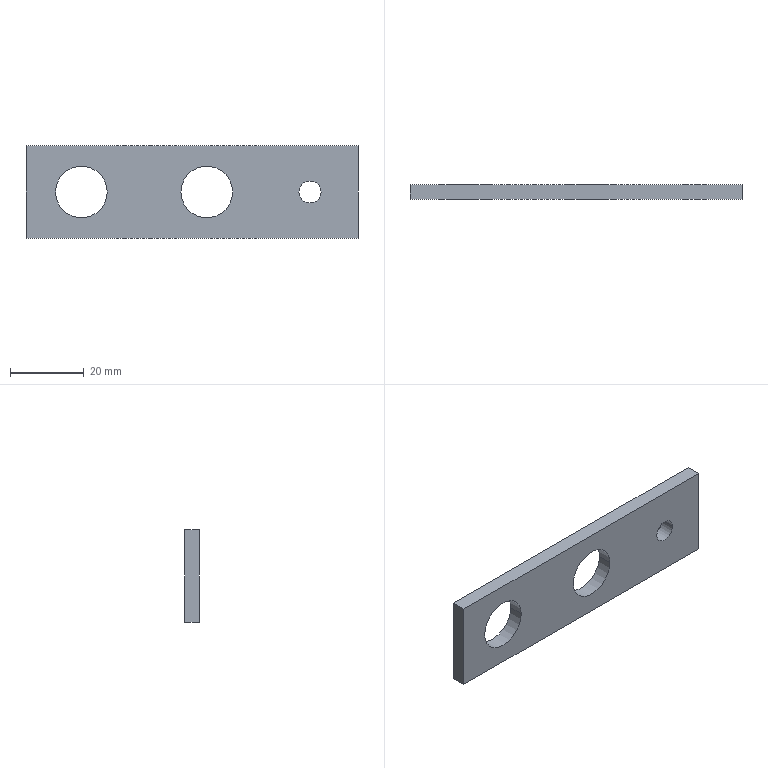Part | STEP file | Connecting plate 2 | 1 solid | 12 faces | box 90 x 4 x 25 mm | volume 7655 mm3 | cylinder 6 | plane 6 | commonest cylinder face diameters 14 x4 6 x2
STEP:
#1=CARTESIAN_POINT('',(-68.,0.,12.5));
#2=VERTEX_POINT('',#1);
#3=CARTESIAN_POINT('',(-82.,0.,12.5));
#4=VERTEX_POINT('',#3);
#5=CARTESIAN_POINT('',(-75.,0.,12.5));
#6=DIRECTION('',(0.,1.,0.));
#7=DIRECTION('',(1.,0.,0.));
#8=AXIS2_PLACEMENT_3D('',#5,#6,#7);
#9=CIRCLE('',#8,7.);
#10=EDGE_CURVE('',#2,#4,#9,.T.);
#11=ORIENTED_EDGE('',*,*,#10,.F.);
#12=CARTESIAN_POINT('',(-68.,4.,12.5));
#13=VERTEX_POINT('',#12);
#14=CARTESIAN_POINT('',(-68.,-0.001,12.5));
#15=DIRECTION('',(0.,1.,0.));
#16=VECTOR('',#15,1000.);
#17=LINE('',#14,#16);
#18=EDGE_CURVE('',#2,#13,#17,.T.);
#19=ORIENTED_EDGE('',*,*,#18,.T.);
#20=CARTESIAN_POINT('',(-82.,4.,12.5));
#21=VERTEX_POINT('',#20);
#22=CARTESIAN_POINT('',(-75.,4.,12.5));
#23=DIRECTION('',(0.,1.,0.));
#24=DIRECTION('',(-1.,0.,0.));
#25=AXIS2_PLACEMENT_3D('',#22,#23,#24);
#26=CIRCLE('',#25,7.);
#27=EDGE_CURVE('',#13,#21,#26,.T.);
#28=ORIENTED_EDGE('',*,*,#27,.T.);
#29=CARTESIAN_POINT('',(-82.,-0.001,12.5));
#30=DIRECTION('',(0.,1.,0.));
#31=VECTOR('',#30,1000.);
#32=LINE('',#29,#31);
#33=EDGE_CURVE('',#4,#21,#32,.T.);
#34=ORIENTED_EDGE('',*,*,#33,.F.);
#35=EDGE_LOOP('',(#11,#19,#28,#34));
#36=FACE_OUTER_BOUND('',#35,.T.);
#37=CARTESIAN_POINT('',(-75.,-0.001,12.5));
#38=DIRECTION('',(0.,1.,0.));
#39=DIRECTION('',(-1.,0.,0.));
#40=AXIS2_PLACEMENT_3D('',#37,#38,#39);
#41=CYLINDRICAL_SURFACE('',#40,7.);
#42=ADVANCED_FACE('',(#36),#41,.F.);
#43=CARTESIAN_POINT('',(-10.,0.,12.5));
#44=VERTEX_POINT('',#43);
#45=CARTESIAN_POINT('',(-16.,0.,12.5));
#46=VERTEX_POINT('',#45);
#47=CARTESIAN_POINT('',(-13.,0.,12.5));
#48=DIRECTION('',(0.,1.,0.));
#49=DIRECTION('',(1.,0.,0.));
#50=AXIS2_PLACEMENT_3D('',#47,#48,#49);
#51=CIRCLE('',#50,3.);
#52=EDGE_CURVE('',#44,#46,#51,.T.);
#53=ORIENTED_EDGE('',*,*,#52,.F.);
#54=CARTESIAN_POINT('',(-10.,4.,12.5));
#55=VERTEX_POINT('',#54);
#56=CARTESIAN_POINT('',(-10.,-0.001,12.5));
#57=DIRECTION('',(0.,1.,0.));
#58=VECTOR('',#57,1000.);
#59=LINE('',#56,#58);
#60=EDGE_CURVE('',#44,#55,#59,.T.);
#61=ORIENTED_EDGE('',*,*,#60,.T.);
#62=CARTESIAN_POINT('',(-16.,4.,12.5));
#63=VERTEX_POINT('',#62);
#64=CARTESIAN_POINT('',(-13.,4.,12.5));
#65=DIRECTION('',(0.,1.,0.));
#66=DIRECTION('',(-1.,0.,0.));
#67=AXIS2_PLACEMENT_3D('',#64,#65,#66);
#68=CIRCLE('',#67,3.);
#69=EDGE_CURVE('',#55,#63,#68,.T.);
#70=ORIENTED_EDGE('',*,*,#69,.T.);
#71=CARTESIAN_POINT('',(-16.,-0.001,12.5));
#72=DIRECTION('',(0.,1.,0.));
#73=VECTOR('',#72,1000.);
#74=LINE('',#71,#73);
#75=EDGE_CURVE('',#46,#63,#74,.T.);
#76=ORIENTED_EDGE('',*,*,#75,.F.);
#77=EDGE_LOOP('',(#53,#61,#70,#76));
#78=FACE_OUTER_BOUND('',#77,.T.);
#79=CARTESIAN_POINT('',(-13.,-0.001,12.5));
#80=DIRECTION('',(0.,1.,0.));
#81=DIRECTION('',(-1.,0.,0.));
#82=AXIS2_PLACEMENT_3D('',#79,#80,#81);
#83=CYLINDRICAL_SURFACE('',#82,3.);
#84=ADVANCED_FACE('',(#78),#83,.F.);
#85=CARTESIAN_POINT('',(-34.,0.,12.5));
#86=VERTEX_POINT('',#85);
#87=CARTESIAN_POINT('',(-48.,0.,12.5));
#88=VERTEX_POINT('',#87);
#89=CARTESIAN_POINT('',(-41.,0.,12.5));
#90=DIRECTION('',(0.,1.,0.));
#91=DIRECTION('',(1.,0.,0.));
#92=AXIS2_PLACEMENT_3D('',#89,#90,#91);
#93=CIRCLE('',#92,7.);
#94=EDGE_CURVE('',#86,#88,#93,.T.);
#95=ORIENTED_EDGE('',*,*,#94,.F.);
#96=CARTESIAN_POINT('',(-34.,4.,12.5));
#97=VERTEX_POINT('',#96);
#98=CARTESIAN_POINT('',(-34.,-0.001,12.5));
#99=DIRECTION('',(0.,1.,0.));
#100=VECTOR('',#99,1000.);
#101=LINE('',#98,#100);
#102=EDGE_CURVE('',#86,#97,#101,.T.);
#103=ORIENTED_EDGE('',*,*,#102,.T.);
#104=CARTESIAN_POINT('',(-48.,4.,12.5));
#105=VERTEX_POINT('',#104);
#106=CARTESIAN_POINT('',(-41.,4.,12.5));
#107=DIRECTION('',(0.,1.,0.));
#108=DIRECTION('',(-1.,0.,0.));
#109=AXIS2_PLACEMENT_3D('',#106,#107,#108);
#110=CIRCLE('',#109,7.);
#111=EDGE_CURVE('',#97,#105,#110,.T.);
#112=ORIENTED_EDGE('',*,*,#111,.T.);
#113=CARTESIAN_POINT('',(-48.,-0.001,12.5));
#114=DIRECTION('',(0.,1.,0.));
#115=VECTOR('',#114,1000.);
#116=LINE('',#113,#115);
#117=EDGE_CURVE('',#88,#105,#116,.T.);
#118=ORIENTED_EDGE('',*,*,#117,.F.);
#119=EDGE_LOOP('',(#95,#103,#112,#118));
#120=FACE_OUTER_BOUND('',#119,.T.);
#121=CARTESIAN_POINT('',(-41.,-0.001,12.5));
#122=DIRECTION('',(0.,1.,0.));
#123=DIRECTION('',(-1.,0.,0.));
#124=AXIS2_PLACEMENT_3D('',#121,#122,#123);
#125=CYLINDRICAL_SURFACE('',#124,7.);
#126=ADVANCED_FACE('',(#120),#125,.F.);
#127=CARTESIAN_POINT('',(-75.,4.,12.5));
#128=DIRECTION('',(0.,1.,0.));
#129=DIRECTION('',(-1.,0.,0.));
#130=AXIS2_PLACEMENT_3D('',#127,#128,#129);
#131=CIRCLE('',#130,7.);
#132=EDGE_CURVE('',#21,#13,#131,.T.);
#133=ORIENTED_EDGE('',*,*,#132,.F.);
#134=ORIENTED_EDGE('',*,*,#27,.F.);
#135=EDGE_LOOP('',(#133,#134));
#136=FACE_BOUND('',#135,.T.);
#137=CARTESIAN_POINT('',(-13.,4.,12.5));
#138=DIRECTION('',(0.,1.,0.));
#139=DIRECTION('',(-1.,0.,0.));
#140=AXIS2_PLACEMENT_3D('',#137,#138,#139);
#141=CIRCLE('',#140,3.);
#142=EDGE_CURVE('',#63,#55,#141,.T.);
#143=ORIENTED_EDGE('',*,*,#142,.F.);
#144=ORIENTED_EDGE('',*,*,#69,.F.);
#145=EDGE_LOOP('',(#143,#144));
#146=FACE_BOUND('',#145,.T.);
#147=CARTESIAN_POINT('',(-41.,4.,12.5));
#148=DIRECTION('',(0.,1.,0.));
#149=DIRECTION('',(-1.,0.,0.));
#150=AXIS2_PLACEMENT_3D('',#147,#148,#149);
#151=CIRCLE('',#150,7.);
#152=EDGE_CURVE('',#105,#97,#151,.T.);
#153=ORIENTED_EDGE('',*,*,#152,.F.);
#154=ORIENTED_EDGE('',*,*,#111,.F.);
#155=EDGE_LOOP('',(#153,#154));
#156=FACE_BOUND('',#155,.T.);
#157=CARTESIAN_POINT('',(0.,4.,0.));
#158=VERTEX_POINT('',#157);
#159=CARTESIAN_POINT('',(-90.,4.,0.));
#160=VERTEX_POINT('',#159);
#161=CARTESIAN_POINT('',(0.,4.,0.));
#162=DIRECTION('',(-1.,0.,0.));
#163=VECTOR('',#162,1000.);
#164=LINE('',#161,#163);
#165=EDGE_CURVE('',#158,#160,#164,.T.);
#166=ORIENTED_EDGE('',*,*,#165,.T.);
#167=CARTESIAN_POINT('',(-90.,4.,25.));
#168=VERTEX_POINT('',#167);
#169=CARTESIAN_POINT('',(-90.,4.,25.));
#170=DIRECTION('',(0.,0.,-1.));
#171=VECTOR('',#170,1000.);
#172=LINE('',#169,#171);
#173=EDGE_CURVE('',#168,#160,#172,.T.);
#174=ORIENTED_EDGE('',*,*,#173,.F.);
#175=CARTESIAN_POINT('',(0.,4.,25.));
#176=VERTEX_POINT('',#175);
#177=CARTESIAN_POINT('',(0.,4.,25.));
#178=DIRECTION('',(-1.,0.,0.));
#179=VECTOR('',#178,1000.);
#180=LINE('',#177,#179);
#181=EDGE_CURVE('',#176,#168,#180,.T.);
#182=ORIENTED_EDGE('',*,*,#181,.F.);
#183=CARTESIAN_POINT('',(0.,4.,25.));
#184=DIRECTION('',(0.,0.,-1.));
#185=VECTOR('',#184,1000.);
#186=LINE('',#183,#185);
#187=EDGE_CURVE('',#176,#158,#186,.T.);
#188=ORIENTED_EDGE('',*,*,#187,.T.);
#189=EDGE_LOOP('',(#166,#174,#182,#188));
#190=FACE_OUTER_BOUND('',#189,.T.);
#191=CARTESIAN_POINT('',(0.,4.,25.));
#192=DIRECTION('',(0.,-1.,0.));
#193=DIRECTION('',(1.,0.,0.));
#194=AXIS2_PLACEMENT_3D('',#191,#192,#193);
#195=PLANE('',#194);
#196=ADVANCED_FACE('',(#136,#146,#156,#190),#195,.F.);
#197=CARTESIAN_POINT('',(-90.,0.,0.));
#198=VERTEX_POINT('',#197);
#199=CARTESIAN_POINT('',(-90.,0.,0.));
#200=DIRECTION('',(0.,1.,0.));
#201=VECTOR('',#200,1000.);
#202=LINE('',#199,#201);
#203=EDGE_CURVE('',#198,#160,#202,.T.);
#204=ORIENTED_EDGE('',*,*,#203,.F.);
#205=CARTESIAN_POINT('',(-90.,0.,25.));
#206=VERTEX_POINT('',#205);
#207=CARTESIAN_POINT('',(-90.,0.,25.));
#208=DIRECTION('',(0.,0.,-1.));
#209=VECTOR('',#208,1000.);
#210=LINE('',#207,#209);
#211=EDGE_CURVE('',#206,#198,#210,.T.);
#212=ORIENTED_EDGE('',*,*,#211,.F.);
#213=CARTESIAN_POINT('',(-90.,0.,25.));
#214=DIRECTION('',(0.,1.,0.));
#215=VECTOR('',#214,1000.);
#216=LINE('',#213,#215);
#217=EDGE_CURVE('',#206,#168,#216,.T.);
#218=ORIENTED_EDGE('',*,*,#217,.T.);
#219=ORIENTED_EDGE('',*,*,#173,.T.);
#220=EDGE_LOOP('',(#204,#212,#218,#219));
#221=FACE_OUTER_BOUND('',#220,.T.);
#222=CARTESIAN_POINT('',(-90.,0.,25.));
#223=DIRECTION('',(-1.,0.,0.));
#224=DIRECTION('',(0.,0.,1.));
#225=AXIS2_PLACEMENT_3D('',#222,#223,#224);
#226=PLANE('',#225);
#227=ADVANCED_FACE('',(#221),#226,.T.);
#228=CARTESIAN_POINT('',(-75.,0.,12.5));
#229=DIRECTION('',(0.,1.,0.));
#230=DIRECTION('',(1.,0.,0.));
#231=AXIS2_PLACEMENT_3D('',#228,#229,#230);
#232=CIRCLE('',#231,7.);
#233=EDGE_CURVE('',#4,#2,#232,.T.);
#234=ORIENTED_EDGE('',*,*,#233,.T.);
#235=ORIENTED_EDGE('',*,*,#10,.T.);
#236=EDGE_LOOP('',(#234,#235));
#237=FACE_BOUND('',#236,.T.);
#238=CARTESIAN_POINT('',(-13.,0.,12.5));
#239=DIRECTION('',(0.,1.,0.));
#240=DIRECTION('',(1.,0.,0.));
#241=AXIS2_PLACEMENT_3D('',#238,#239,#240);
#242=CIRCLE('',#241,3.);
#243=EDGE_CURVE('',#46,#44,#242,.T.);
#244=ORIENTED_EDGE('',*,*,#243,.T.);
#245=ORIENTED_EDGE('',*,*,#52,.T.);
#246=EDGE_LOOP('',(#244,#245));
#247=FACE_BOUND('',#246,.T.);
#248=CARTESIAN_POINT('',(-41.,0.,12.5));
#249=DIRECTION('',(0.,1.,0.));
#250=DIRECTION('',(1.,0.,0.));
#251=AXIS2_PLACEMENT_3D('',#248,#249,#250);
#252=CIRCLE('',#251,7.);
#253=EDGE_CURVE('',#88,#86,#252,.T.);
#254=ORIENTED_EDGE('',*,*,#253,.T.);
#255=ORIENTED_EDGE('',*,*,#94,.T.);
#256=EDGE_LOOP('',(#254,#255));
#257=FACE_BOUND('',#256,.T.);
#258=CARTESIAN_POINT('',(0.,0.,0.));
#259=VERTEX_POINT('',#258);
#260=CARTESIAN_POINT('',(0.,0.,0.));
#261=DIRECTION('',(-1.,0.,0.));
#262=VECTOR('',#261,1000.);
#263=LINE('',#260,#262);
#264=EDGE_CURVE('',#259,#198,#263,.T.);
#265=ORIENTED_EDGE('',*,*,#264,.F.);
#266=CARTESIAN_POINT('',(0.,0.,25.));
#267=VERTEX_POINT('',#266);
#268=CARTESIAN_POINT('',(0.,0.,25.));
#269=DIRECTION('',(0.,0.,-1.));
#270=VECTOR('',#269,1000.);
#271=LINE('',#268,#270);
#272=EDGE_CURVE('',#267,#259,#271,.T.);
#273=ORIENTED_EDGE('',*,*,#272,.F.);
#274=CARTESIAN_POINT('',(0.,0.,25.));
#275=DIRECTION('',(-1.,0.,0.));
#276=VECTOR('',#275,1000.);
#277=LINE('',#274,#276);
#278=EDGE_CURVE('',#267,#206,#277,.T.);
#279=ORIENTED_EDGE('',*,*,#278,.T.);
#280=ORIENTED_EDGE('',*,*,#211,.T.);
#281=EDGE_LOOP('',(#265,#273,#279,#280));
#282=FACE_OUTER_BOUND('',#281,.T.);
#283=CARTESIAN_POINT('',(0.,0.,25.));
#284=DIRECTION('',(0.,-1.,0.));
#285=DIRECTION('',(1.,0.,0.));
#286=AXIS2_PLACEMENT_3D('',#283,#284,#285);
#287=PLANE('',#286);
#288=ADVANCED_FACE('',(#237,#247,#257,#282),#287,.T.);
#289=CARTESIAN_POINT('',(0.,4.,0.));
#290=DIRECTION('',(0.,-1.,0.));
#291=VECTOR('',#290,1000.);
#292=LINE('',#289,#291);
#293=EDGE_CURVE('',#158,#259,#292,.T.);
#294=ORIENTED_EDGE('',*,*,#293,.F.);
#295=ORIENTED_EDGE('',*,*,#187,.F.);
#296=CARTESIAN_POINT('',(0.,4.,25.));
#297=DIRECTION('',(0.,-1.,0.));
#298=VECTOR('',#297,1000.);
#299=LINE('',#296,#298);
#300=EDGE_CURVE('',#176,#267,#299,.T.);
#301=ORIENTED_EDGE('',*,*,#300,.T.);
#302=ORIENTED_EDGE('',*,*,#272,.T.);
#303=EDGE_LOOP('',(#294,#295,#301,#302));
#304=FACE_OUTER_BOUND('',#303,.T.);
#305=CARTESIAN_POINT('',(0.,4.,25.));
#306=DIRECTION('',(1.,0.,0.));
#307=DIRECTION('',(0.,1.,0.));
#308=AXIS2_PLACEMENT_3D('',#305,#306,#307);
#309=PLANE('',#308);
#310=ADVANCED_FACE('',(#304),#309,.T.);
#311=ORIENTED_EDGE('',*,*,#181,.T.);
#312=ORIENTED_EDGE('',*,*,#217,.F.);
#313=ORIENTED_EDGE('',*,*,#278,.F.);
#314=ORIENTED_EDGE('',*,*,#300,.F.);
#315=EDGE_LOOP('',(#311,#312,#313,#314));
#316=FACE_OUTER_BOUND('',#315,.T.);
#317=CARTESIAN_POINT('',(0.,0.,25.));
#318=DIRECTION('',(0.,0.,-1.));
#319=DIRECTION('',(-1.,0.,0.));
#320=AXIS2_PLACEMENT_3D('',#317,#318,#319);
#321=PLANE('',#320);
#322=ADVANCED_FACE('',(#316),#321,.F.);
#323=ORIENTED_EDGE('',*,*,#165,.F.);
#324=ORIENTED_EDGE('',*,*,#293,.T.);
#325=ORIENTED_EDGE('',*,*,#264,.T.);
#326=ORIENTED_EDGE('',*,*,#203,.T.);
#327=EDGE_LOOP('',(#323,#324,#325,#326));
#328=FACE_OUTER_BOUND('',#327,.T.);
#329=CARTESIAN_POINT('',(0.,0.,0.));
#330=DIRECTION('',(0.,0.,-1.));
#331=DIRECTION('',(-1.,0.,0.));
#332=AXIS2_PLACEMENT_3D('',#329,#330,#331);
#333=PLANE('',#332);
#334=ADVANCED_FACE('',(#328),#333,.T.);
#335=ORIENTED_EDGE('',*,*,#102,.F.);
#336=ORIENTED_EDGE('',*,*,#253,.F.);
#337=ORIENTED_EDGE('',*,*,#117,.T.);
#338=ORIENTED_EDGE('',*,*,#152,.T.);
#339=EDGE_LOOP('',(#335,#336,#337,#338));
#340=FACE_OUTER_BOUND('',#339,.T.);
#341=CARTESIAN_POINT('',(-41.,-0.001,12.5));
#342=DIRECTION('',(0.,1.,0.));
#343=DIRECTION('',(-1.,0.,0.));
#344=AXIS2_PLACEMENT_3D('',#341,#342,#343);
#345=CYLINDRICAL_SURFACE('',#344,7.);
#346=ADVANCED_FACE('',(#340),#345,.F.);
#347=ORIENTED_EDGE('',*,*,#60,.F.);
#348=ORIENTED_EDGE('',*,*,#243,.F.);
#349=ORIENTED_EDGE('',*,*,#75,.T.);
#350=ORIENTED_EDGE('',*,*,#142,.T.);
#351=EDGE_LOOP('',(#347,#348,#349,#350));
#352=FACE_OUTER_BOUND('',#351,.T.);
#353=CARTESIAN_POINT('',(-13.,-0.001,12.5));
#354=DIRECTION('',(0.,1.,0.));
#355=DIRECTION('',(-1.,0.,0.));
#356=AXIS2_PLACEMENT_3D('',#353,#354,#355);
#357=CYLINDRICAL_SURFACE('',#356,3.);
#358=ADVANCED_FACE('',(#352),#357,.F.);
#359=ORIENTED_EDGE('',*,*,#18,.F.);
#360=ORIENTED_EDGE('',*,*,#233,.F.);
#361=ORIENTED_EDGE('',*,*,#33,.T.);
#362=ORIENTED_EDGE('',*,*,#132,.T.);
#363=EDGE_LOOP('',(#359,#360,#361,#362));
#364=FACE_OUTER_BOUND('',#363,.T.);
#365=CARTESIAN_POINT('',(-75.,-0.001,12.5));
#366=DIRECTION('',(0.,1.,0.));
#367=DIRECTION('',(-1.,0.,0.));
#368=AXIS2_PLACEMENT_3D('',#365,#366,#367);
#369=CYLINDRICAL_SURFACE('',#368,7.);
#370=ADVANCED_FACE('',(#364),#369,.F.);
#371=CLOSED_SHELL('',(#42,#84,#126,#196,#227,#288,#310,#322,#334,#346,#358,#370));
#372=MANIFOLD_SOLID_BREP('',#371);
#373=CARTESIAN_POINT('',(0.,0.,0.));
#374=DIRECTION('',(0.,0.,1.));
#375=DIRECTION('',(1.,0.,0.));
#376=AXIS2_PLACEMENT_3D('',#373,#374,#375);
#377=(LENGTH_UNIT()NAMED_UNIT(*)SI_UNIT(.MILLI.,.METRE.));
#378=UNCERTAINTY_MEASURE_WITH_UNIT(LENGTH_MEASURE(0.00001),#377,'','');
#379=(NAMED_UNIT(*)PLANE_ANGLE_UNIT()SI_UNIT($,.RADIAN.));
#380=(NAMED_UNIT(*)SI_UNIT($,.STERADIAN.)SOLID_ANGLE_UNIT());
#381=(GEOMETRIC_REPRESENTATION_CONTEXT(3)GLOBAL_UNCERTAINTY_ASSIGNED_CONTEXT((#378))GLOBAL_UNIT_ASSIGNED_CONTEXT((#377,#379,#380))REPRESENTATION_CONTEXT('',''));
#382=ADVANCED_BREP_SHAPE_REPRESENTATION('',(#372,#376),#381);